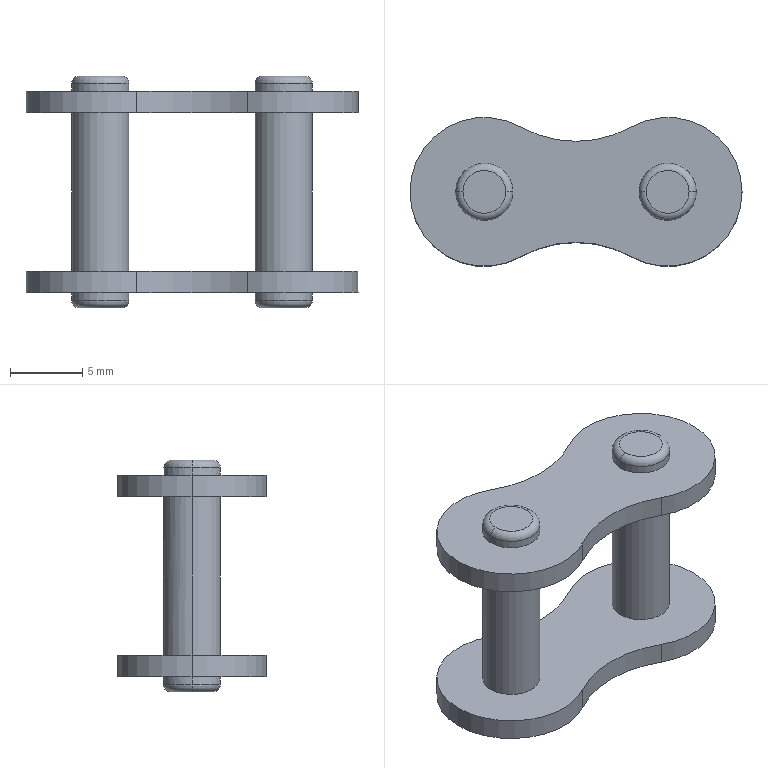Part | STEP file | _CHE40-500_c1 | 1 solid | 40 faces | box 23 x 10.3 x 16.04 mm | volume 895.191 mm3 | cylinder 24 | plane 8 | torus 8 | commonest cylinder face diameters 3.97 x12 10.3 x8 15.788 x4
STEP:
#1=CARTESIAN_POINT('',(2.507,4.499,-5.475));
#2=VERTEX_POINT('',#1);
#3=CARTESIAN_POINT('',(10.193,4.499,-5.475));
#4=VERTEX_POINT('',#3);
#5=CARTESIAN_POINT('',(6.35,11.394,-5.475));
#6=DIRECTION('',(0.,0.,1.));
#7=AXIS2_PLACEMENT_3D('',#5,#6,$);
#8=CIRCLE('',#7,7.894);
#9=EDGE_CURVE('',#2,#4,#8,.T.);
#10=ORIENTED_EDGE('',*,*,#9,.F.);
#11=CARTESIAN_POINT('',(-5.15,0.,-5.475));
#12=VERTEX_POINT('',#11);
#13=CARTESIAN_POINT('',(0.,0.,-5.475));
#14=DIRECTION('',(0.,0.,1.));
#15=AXIS2_PLACEMENT_3D('',#13,#14,$);
#16=CIRCLE('',#15,5.15);
#17=EDGE_CURVE('',#2,#12,#16,.T.);
#18=ORIENTED_EDGE('',*,*,#17,.T.);
#19=CARTESIAN_POINT('',(2.507,-4.499,-5.475));
#20=VERTEX_POINT('',#19);
#21=CARTESIAN_POINT('',(0.,0.,-5.475));
#22=DIRECTION('',(0.,0.,1.));
#23=AXIS2_PLACEMENT_3D('',#21,#22,$);
#24=CIRCLE('',#23,5.15);
#25=EDGE_CURVE('',#12,#20,#24,.T.);
#26=ORIENTED_EDGE('',*,*,#25,.T.);
#27=CARTESIAN_POINT('',(10.193,-4.499,-5.475));
#28=VERTEX_POINT('',#27);
#29=CARTESIAN_POINT('',(6.35,-11.394,-5.475));
#30=DIRECTION('',(0.,0.,1.));
#31=AXIS2_PLACEMENT_3D('',#29,#30,$);
#32=CIRCLE('',#31,7.894);
#33=EDGE_CURVE('',#28,#20,#32,.T.);
#34=ORIENTED_EDGE('',*,*,#33,.F.);
#35=CARTESIAN_POINT('',(17.85,0.,-5.475));
#36=VERTEX_POINT('',#35);
#37=CARTESIAN_POINT('',(12.7,0.,-5.475));
#38=DIRECTION('',(0.,0.,1.));
#39=AXIS2_PLACEMENT_3D('',#37,#38,$);
#40=CIRCLE('',#39,5.15);
#41=EDGE_CURVE('',#28,#36,#40,.T.);
#42=ORIENTED_EDGE('',*,*,#41,.T.);
#43=CARTESIAN_POINT('',(12.7,0.,-5.475));
#44=DIRECTION('',(0.,0.,1.));
#45=AXIS2_PLACEMENT_3D('',#43,#44,$);
#46=CIRCLE('',#45,5.15);
#47=EDGE_CURVE('',#36,#4,#46,.T.);
#48=ORIENTED_EDGE('',*,*,#47,.T.);
#49=EDGE_LOOP('',(#10,#18,#26,#34,#42,#48));
#50=FACE_OUTER_BOUND('',#49,.T.);
#51=CARTESIAN_POINT('',(-1.985,0.000000001,-5.475));
#52=VERTEX_POINT('',#51);
#53=CARTESIAN_POINT('',(1.985,0.000000001,-5.475));
#54=VERTEX_POINT('',#53);
#55=CARTESIAN_POINT('',(0.000000001,0.,-5.475));
#56=DIRECTION('',(0.,0.,1.));
#57=AXIS2_PLACEMENT_3D('',#55,#56,$);
#58=CIRCLE('',#57,1.985);
#59=EDGE_CURVE('',#52,#54,#58,.T.);
#60=ORIENTED_EDGE('',*,*,#59,.F.);
#61=CARTESIAN_POINT('',(0.000000001,0.,-5.475));
#62=DIRECTION('',(0.,0.,1.));
#63=AXIS2_PLACEMENT_3D('',#61,#62,$);
#64=CIRCLE('',#63,1.985);
#65=EDGE_CURVE('',#54,#52,#64,.T.);
#66=ORIENTED_EDGE('',*,*,#65,.F.);
#67=EDGE_LOOP('',(#60,#66));
#68=FACE_BOUND('',#67,.T.);
#69=CARTESIAN_POINT('',(10.715,0.000000001,-5.475));
#70=VERTEX_POINT('',#69);
#71=CARTESIAN_POINT('',(14.685,0.000000001,-5.475));
#72=VERTEX_POINT('',#71);
#73=CARTESIAN_POINT('',(12.7,0.,-5.475));
#74=DIRECTION('',(0.,0.,1.));
#75=AXIS2_PLACEMENT_3D('',#73,#74,$);
#76=CIRCLE('',#75,1.985);
#77=EDGE_CURVE('',#70,#72,#76,.T.);
#78=ORIENTED_EDGE('',*,*,#77,.F.);
#79=CARTESIAN_POINT('',(12.7,0.,-5.475));
#80=DIRECTION('',(0.,0.,1.));
#81=AXIS2_PLACEMENT_3D('',#79,#80,$);
#82=CIRCLE('',#81,1.985);
#83=EDGE_CURVE('',#72,#70,#82,.T.);
#84=ORIENTED_EDGE('',*,*,#83,.F.);
#85=EDGE_LOOP('',(#78,#84));
#86=FACE_BOUND('',#85,.T.);
#87=CARTESIAN_POINT('',(9.525,5.697,-5.475));
#88=DIRECTION('',(0.,0.,1.));
#89=DIRECTION('',(1.,0.,0.));
#90=AXIS2_PLACEMENT_3D('',#87,#88,#89);
#91=PLANE('',#90);
#92=ADVANCED_FACE('',(#50,#68,#86),#91,.T.);
#93=ORIENTED_EDGE('',*,*,#9,.T.);
#94=CARTESIAN_POINT('',(10.193,4.499,-6.975));
#95=VERTEX_POINT('',#94);
#96=CARTESIAN_POINT('',(10.193,4.499,-6.975));
#97=DIRECTION('',(0.,0.,-1.));
#98=VECTOR('',#97,1.);
#99=LINE('',#96,#98);
#100=EDGE_CURVE('',#95,#4,#99,.F.);
#101=ORIENTED_EDGE('',*,*,#100,.F.);
#102=CARTESIAN_POINT('',(2.507,4.499,-6.975));
#103=VERTEX_POINT('',#102);
#104=CARTESIAN_POINT('',(6.35,11.394,-6.975));
#105=DIRECTION('',(0.,0.,-1.));
#106=AXIS2_PLACEMENT_3D('',#104,#105,$);
#107=CIRCLE('',#106,7.894);
#108=EDGE_CURVE('',#103,#95,#107,.F.);
#109=ORIENTED_EDGE('',*,*,#108,.F.);
#110=CARTESIAN_POINT('',(2.507,4.499,-6.975));
#111=DIRECTION('',(0.,0.,-1.));
#112=VECTOR('',#111,1.);
#113=LINE('',#110,#112);
#114=EDGE_CURVE('',#103,#2,#113,.F.);
#115=ORIENTED_EDGE('',*,*,#114,.T.);
#116=EDGE_LOOP('',(#93,#101,#109,#115));
#117=FACE_OUTER_BOUND('',#116,.T.);
#118=CARTESIAN_POINT('',(6.35,11.394,-6.975));
#119=DIRECTION('',(0.,0.,-1.));
#120=DIRECTION('',(1.,0.,0.));
#121=AXIS2_PLACEMENT_3D('',#118,#119,#120);
#122=CYLINDRICAL_SURFACE('',#121,7.894);
#123=ADVANCED_FACE('',(#117),#122,.F.);
#124=CARTESIAN_POINT('',(-5.15,0.,-6.975));
#125=VERTEX_POINT('',#124);
#126=CARTESIAN_POINT('',(-5.15,0.,-6.975));
#127=DIRECTION('',(0.,0.,-1.));
#128=VECTOR('',#127,1.);
#129=LINE('',#126,#128);
#130=EDGE_CURVE('',#12,#125,#129,.T.);
#131=ORIENTED_EDGE('',*,*,#130,.F.);
#132=ORIENTED_EDGE('',*,*,#17,.F.);
#133=ORIENTED_EDGE('',*,*,#114,.F.);
#134=CARTESIAN_POINT('',(0.,0.,-6.975));
#135=DIRECTION('',(0.,0.,-1.));
#136=AXIS2_PLACEMENT_3D('',#134,#135,$);
#137=CIRCLE('',#136,5.15);
#138=EDGE_CURVE('',#103,#125,#137,.F.);
#139=ORIENTED_EDGE('',*,*,#138,.T.);
#140=EDGE_LOOP('',(#131,#132,#133,#139));
#141=FACE_OUTER_BOUND('',#140,.T.);
#142=CARTESIAN_POINT('',(0.,0.,-6.975));
#143=DIRECTION('',(0.,0.,-1.));
#144=DIRECTION('',(-1.,0.,0.));
#145=AXIS2_PLACEMENT_3D('',#142,#143,#144);
#146=CYLINDRICAL_SURFACE('',#145,5.15);
#147=ADVANCED_FACE('',(#141),#146,.T.);
#148=ORIENTED_EDGE('',*,*,#130,.T.);
#149=CARTESIAN_POINT('',(2.507,-4.499,-6.975));
#150=VERTEX_POINT('',#149);
#151=CARTESIAN_POINT('',(0.,0.,-6.975));
#152=DIRECTION('',(0.,0.,-1.));
#153=AXIS2_PLACEMENT_3D('',#151,#152,$);
#154=CIRCLE('',#153,5.15);
#155=EDGE_CURVE('',#125,#150,#154,.F.);
#156=ORIENTED_EDGE('',*,*,#155,.T.);
#157=CARTESIAN_POINT('',(2.507,-4.499,-6.975));
#158=DIRECTION('',(0.,0.,-1.));
#159=VECTOR('',#158,1.);
#160=LINE('',#157,#159);
#161=EDGE_CURVE('',#150,#20,#160,.F.);
#162=ORIENTED_EDGE('',*,*,#161,.T.);
#163=ORIENTED_EDGE('',*,*,#25,.F.);
#164=EDGE_LOOP('',(#148,#156,#162,#163));
#165=FACE_OUTER_BOUND('',#164,.T.);
#166=CARTESIAN_POINT('',(0.,0.,-6.975));
#167=DIRECTION('',(0.,0.,-1.));
#168=DIRECTION('',(1.,0.,0.));
#169=AXIS2_PLACEMENT_3D('',#166,#167,#168);
#170=CYLINDRICAL_SURFACE('',#169,5.15);
#171=ADVANCED_FACE('',(#165),#170,.T.);
#172=ORIENTED_EDGE('',*,*,#33,.T.);
#173=ORIENTED_EDGE('',*,*,#161,.F.);
#174=CARTESIAN_POINT('',(10.193,-4.499,-6.975));
#175=VERTEX_POINT('',#174);
#176=CARTESIAN_POINT('',(6.35,-11.394,-6.975));
#177=DIRECTION('',(0.,0.,-1.));
#178=AXIS2_PLACEMENT_3D('',#176,#177,$);
#179=CIRCLE('',#178,7.894);
#180=EDGE_CURVE('',#175,#150,#179,.F.);
#181=ORIENTED_EDGE('',*,*,#180,.F.);
#182=CARTESIAN_POINT('',(10.193,-4.499,-6.975));
#183=DIRECTION('',(0.,0.,-1.));
#184=VECTOR('',#183,1.);
#185=LINE('',#182,#184);
#186=EDGE_CURVE('',#175,#28,#185,.F.);
#187=ORIENTED_EDGE('',*,*,#186,.T.);
#188=EDGE_LOOP('',(#172,#173,#181,#187));
#189=FACE_OUTER_BOUND('',#188,.T.);
#190=CARTESIAN_POINT('',(6.35,-11.394,-6.975));
#191=DIRECTION('',(0.,0.,-1.));
#192=DIRECTION('',(-1.,0.,0.));
#193=AXIS2_PLACEMENT_3D('',#190,#191,#192);
#194=CYLINDRICAL_SURFACE('',#193,7.894);
#195=ADVANCED_FACE('',(#189),#194,.F.);
#196=CARTESIAN_POINT('',(17.85,0.,-6.975));
#197=VERTEX_POINT('',#196);
#198=CARTESIAN_POINT('',(17.85,0.,-6.975));
#199=DIRECTION('',(0.,0.,-1.));
#200=VECTOR('',#199,1.);
#201=LINE('',#198,#200);
#202=EDGE_CURVE('',#197,#36,#201,.F.);
#203=ORIENTED_EDGE('',*,*,#202,.T.);
#204=ORIENTED_EDGE('',*,*,#41,.F.);
#205=ORIENTED_EDGE('',*,*,#186,.F.);
#206=CARTESIAN_POINT('',(12.7,0.,-6.975));
#207=DIRECTION('',(0.,0.,-1.));
#208=AXIS2_PLACEMENT_3D('',#206,#207,$);
#209=CIRCLE('',#208,5.15);
#210=EDGE_CURVE('',#175,#197,#209,.F.);
#211=ORIENTED_EDGE('',*,*,#210,.T.);
#212=EDGE_LOOP('',(#203,#204,#205,#211));
#213=FACE_OUTER_BOUND('',#212,.T.);
#214=CARTESIAN_POINT('',(12.7,0.,-6.975));
#215=DIRECTION('',(0.,0.,-1.));
#216=DIRECTION('',(1.,0.,0.));
#217=AXIS2_PLACEMENT_3D('',#214,#215,#216);
#218=CYLINDRICAL_SURFACE('',#217,5.15);
#219=ADVANCED_FACE('',(#213),#218,.T.);
#220=ORIENTED_EDGE('',*,*,#202,.F.);
#221=CARTESIAN_POINT('',(12.7,0.,-6.975));
#222=DIRECTION('',(0.,0.,-1.));
#223=AXIS2_PLACEMENT_3D('',#221,#222,$);
#224=CIRCLE('',#223,5.15);
#225=EDGE_CURVE('',#197,#95,#224,.F.);
#226=ORIENTED_EDGE('',*,*,#225,.T.);
#227=ORIENTED_EDGE('',*,*,#100,.T.);
#228=ORIENTED_EDGE('',*,*,#47,.F.);
#229=EDGE_LOOP('',(#220,#226,#227,#228));
#230=FACE_OUTER_BOUND('',#229,.T.);
#231=CARTESIAN_POINT('',(12.7,0.,-6.975));
#232=DIRECTION('',(0.,0.,-1.));
#233=DIRECTION('',(-1.,0.,0.));
#234=AXIS2_PLACEMENT_3D('',#231,#232,#233);
#235=CYLINDRICAL_SURFACE('',#234,5.15);
#236=ADVANCED_FACE('',(#230),#235,.T.);
#237=CARTESIAN_POINT('',(-1.985,0.000000001,5.475));
#238=VERTEX_POINT('',#237);
#239=CARTESIAN_POINT('',(-1.985,0.,8.02));
#240=DIRECTION('',(0.,0.,-1.));
#241=VECTOR('',#240,1.);
#242=LINE('',#239,#241);
#243=EDGE_CURVE('',#238,#52,#242,.T.);
#244=ORIENTED_EDGE('',*,*,#243,.T.);
#245=ORIENTED_EDGE('',*,*,#59,.T.);
#246=CARTESIAN_POINT('',(1.985,0.000000001,5.475));
#247=VERTEX_POINT('',#246);
#248=CARTESIAN_POINT('',(1.985,0.,8.02));
#249=DIRECTION('',(0.,0.,-1.));
#250=VECTOR('',#249,1.);
#251=LINE('',#248,#250);
#252=EDGE_CURVE('',#54,#247,#251,.F.);
#253=ORIENTED_EDGE('',*,*,#252,.T.);
#254=CARTESIAN_POINT('',(0.,0.,5.475));
#255=DIRECTION('',(0.,0.,-1.));
#256=AXIS2_PLACEMENT_3D('',#254,#255,$);
#257=CIRCLE('',#256,1.985);
#258=EDGE_CURVE('',#247,#238,#257,.T.);
#259=ORIENTED_EDGE('',*,*,#258,.T.);
#260=EDGE_LOOP('',(#244,#245,#253,#259));
#261=FACE_OUTER_BOUND('',#260,.T.);
#262=CARTESIAN_POINT('',(0.,0.,8.02));
#263=DIRECTION('',(0.,0.,-1.));
#264=DIRECTION('',(1.,0.,0.));
#265=AXIS2_PLACEMENT_3D('',#262,#263,#264);
#266=CYLINDRICAL_SURFACE('',#265,1.985);
#267=ADVANCED_FACE('',(#261),#266,.T.);
#268=ORIENTED_EDGE('',*,*,#252,.F.);
#269=ORIENTED_EDGE('',*,*,#65,.T.);
#270=ORIENTED_EDGE('',*,*,#243,.F.);
#271=CARTESIAN_POINT('',(1.985,0.,5.475));
#272=CARTESIAN_POINT('',(1.985,0.6236,5.475));
#273=CARTESIAN_POINT('',(1.74,1.247,5.475));
#274=CARTESIAN_POINT('',(1.247,1.74,5.475));
#275=CARTESIAN_POINT('',(0.,2.23,5.475));
#276=CARTESIAN_POINT('',(-1.247,1.74,5.475));
#277=CARTESIAN_POINT('',(-1.74,1.247,5.475));
#278=CARTESIAN_POINT('',(-1.985,0.6236,5.475));
#279=CARTESIAN_POINT('',(-1.985,0.,5.475));
#280=B_SPLINE_CURVE_WITH_KNOTS('',5,(#271,#272,#273,#274,#275,#276,#277,#278,#279),.UNSPECIFIED.,.F.,.U.,(6,3,6),(-3.118,0.,3.118),.UNSPECIFIED.);
#281=EDGE_CURVE('',#238,#247,#280,.F.);
#282=ORIENTED_EDGE('',*,*,#281,.T.);
#283=EDGE_LOOP('',(#268,#269,#270,#282));
#284=FACE_OUTER_BOUND('',#283,.T.);
#285=CARTESIAN_POINT('',(0.,0.,8.02));
#286=DIRECTION('',(0.,0.,-1.));
#287=DIRECTION('',(-1.,0.,0.));
#288=AXIS2_PLACEMENT_3D('',#285,#286,#287);
#289=CYLINDRICAL_SURFACE('',#288,1.985);
#290=ADVANCED_FACE('',(#284),#289,.T.);
#291=CARTESIAN_POINT('',(10.715,0.000000001,5.475));
#292=VERTEX_POINT('',#291);
#293=CARTESIAN_POINT('',(10.715,0.,8.02));
#294=DIRECTION('',(0.,0.,-1.));
#295=VECTOR('',#294,1.);
#296=LINE('',#293,#295);
#297=EDGE_CURVE('',#292,#70,#296,.T.);
#298=ORIENTED_EDGE('',*,*,#297,.T.);
#299=ORIENTED_EDGE('',*,*,#77,.T.);
#300=CARTESIAN_POINT('',(14.685,0.000000001,5.475));
#301=VERTEX_POINT('',#300);
#302=CARTESIAN_POINT('',(14.685,0.,8.02));
#303=DIRECTION('',(0.,0.,-1.));
#304=VECTOR('',#303,1.);
#305=LINE('',#302,#304);
#306=EDGE_CURVE('',#72,#301,#305,.F.);
#307=ORIENTED_EDGE('',*,*,#306,.T.);
#308=CARTESIAN_POINT('',(12.7,0.,5.475));
#309=DIRECTION('',(0.,0.,-1.));
#310=AXIS2_PLACEMENT_3D('',#308,#309,$);
#311=CIRCLE('',#310,1.985);
#312=EDGE_CURVE('',#301,#292,#311,.T.);
#313=ORIENTED_EDGE('',*,*,#312,.T.);
#314=EDGE_LOOP('',(#298,#299,#307,#313));
#315=FACE_OUTER_BOUND('',#314,.T.);
#316=CARTESIAN_POINT('',(12.7,0.,8.02));
#317=DIRECTION('',(0.,0.,-1.));
#318=DIRECTION('',(1.,0.,0.));
#319=AXIS2_PLACEMENT_3D('',#316,#317,#318);
#320=CYLINDRICAL_SURFACE('',#319,1.985);
#321=ADVANCED_FACE('',(#315),#320,.T.);
#322=ORIENTED_EDGE('',*,*,#306,.F.);
#323=ORIENTED_EDGE('',*,*,#83,.T.);
#324=ORIENTED_EDGE('',*,*,#297,.F.);
#325=CARTESIAN_POINT('',(14.685,0.,5.475));
#326=CARTESIAN_POINT('',(14.685,0.6236,5.475));
#327=CARTESIAN_POINT('',(14.44,1.247,5.475));
#328=CARTESIAN_POINT('',(13.947,1.74,5.475));
#329=CARTESIAN_POINT('',(12.7,2.23,5.475));
#330=CARTESIAN_POINT('',(11.453,1.74,5.475));
#331=CARTESIAN_POINT('',(10.96,1.247,5.475));
#332=CARTESIAN_POINT('',(10.715,0.6236,5.475));
#333=CARTESIAN_POINT('',(10.715,0.,5.475));
#334=B_SPLINE_CURVE_WITH_KNOTS('',5,(#325,#326,#327,#328,#329,#330,#331,#332,#333),.UNSPECIFIED.,.F.,.U.,(6,3,6),(-3.118,0.,3.118),.UNSPECIFIED.);
#335=EDGE_CURVE('',#292,#301,#334,.F.);
#336=ORIENTED_EDGE('',*,*,#335,.T.);
#337=EDGE_LOOP('',(#322,#323,#324,#336));
#338=FACE_OUTER_BOUND('',#337,.T.);
#339=CARTESIAN_POINT('',(12.7,0.,8.02));
#340=DIRECTION('',(0.,0.,-1.));
#341=DIRECTION('',(-1.,0.,0.));
#342=AXIS2_PLACEMENT_3D('',#339,#340,#341);
#343=CYLINDRICAL_SURFACE('',#342,1.985);
#344=ADVANCED_FACE('',(#338),#343,.T.);
#345=ORIENTED_EDGE('',*,*,#108,.T.);
#346=ORIENTED_EDGE('',*,*,#225,.F.);
#347=ORIENTED_EDGE('',*,*,#210,.F.);
#348=ORIENTED_EDGE('',*,*,#180,.T.);
#349=ORIENTED_EDGE('',*,*,#155,.F.);
#350=ORIENTED_EDGE('',*,*,#138,.F.);
#351=EDGE_LOOP('',(#345,#346,#347,#348,#349,#350));
#352=FACE_OUTER_BOUND('',#351,.T.);
#353=CARTESIAN_POINT('',(1.985,0.,-6.975));
#354=VERTEX_POINT('',#353);
#355=CARTESIAN_POINT('',(-1.985,0.,-6.975));
#356=VERTEX_POINT('',#355);
#357=CARTESIAN_POINT('',(0.000000001,0.,-6.975));
#358=DIRECTION('',(0.,0.,1.));
#359=AXIS2_PLACEMENT_3D('',#357,#358,$);
#360=CIRCLE('',#359,1.985);
#361=EDGE_CURVE('',#354,#356,#360,.T.);
#362=ORIENTED_EDGE('',*,*,#361,.T.);
#363=CARTESIAN_POINT('',(0.000000001,0.,-6.975));
#364=DIRECTION('',(0.,0.,1.));
#365=AXIS2_PLACEMENT_3D('',#363,#364,$);
#366=CIRCLE('',#365,1.985);
#367=EDGE_CURVE('',#356,#354,#366,.T.);
#368=ORIENTED_EDGE('',*,*,#367,.T.);
#369=EDGE_LOOP('',(#362,#368));
#370=FACE_BOUND('',#369,.T.);
#371=CARTESIAN_POINT('',(14.685,0.000000001,-6.975));
#372=VERTEX_POINT('',#371);
#373=CARTESIAN_POINT('',(10.715,0.000000001,-6.975));
#374=VERTEX_POINT('',#373);
#375=CARTESIAN_POINT('',(12.7,0.,-6.975));
#376=DIRECTION('',(0.,0.,1.));
#377=AXIS2_PLACEMENT_3D('',#375,#376,$);
#378=CIRCLE('',#377,1.985);
#379=EDGE_CURVE('',#372,#374,#378,.T.);
#380=ORIENTED_EDGE('',*,*,#379,.T.);
#381=CARTESIAN_POINT('',(12.7,0.,-6.975));
#382=DIRECTION('',(0.,0.,1.));
#383=AXIS2_PLACEMENT_3D('',#381,#382,$);
#384=CIRCLE('',#383,1.985);
#385=EDGE_CURVE('',#374,#372,#384,.T.);
#386=ORIENTED_EDGE('',*,*,#385,.T.);
#387=EDGE_LOOP('',(#380,#386));
#388=FACE_BOUND('',#387,.T.);
#389=CARTESIAN_POINT('',(9.525,5.697,-6.975));
#390=DIRECTION('',(0.,0.,1.));
#391=DIRECTION('',(1.,0.,0.));
#392=AXIS2_PLACEMENT_3D('',#389,#390,#391);
#393=PLANE('',#392);
#394=ADVANCED_FACE('',(#352,#370,#388),#393,.F.);
#395=CARTESIAN_POINT('',(2.507,4.499,5.475));
#396=VERTEX_POINT('',#395);
#397=CARTESIAN_POINT('',(10.193,4.499,5.475));
#398=VERTEX_POINT('',#397);
#399=CARTESIAN_POINT('',(6.35,11.394,5.475));
#400=DIRECTION('',(0.,0.,1.));
#401=AXIS2_PLACEMENT_3D('',#399,#400,$);
#402=CIRCLE('',#401,7.894);
#403=EDGE_CURVE('',#396,#398,#402,.T.);
#404=ORIENTED_EDGE('',*,*,#403,.T.);
#405=CARTESIAN_POINT('',(17.85,0.,5.475));
#406=VERTEX_POINT('',#405);
#407=CARTESIAN_POINT('',(12.7,0.,5.475));
#408=DIRECTION('',(0.,0.,1.));
#409=AXIS2_PLACEMENT_3D('',#407,#408,$);
#410=CIRCLE('',#409,5.15);
#411=EDGE_CURVE('',#406,#398,#410,.T.);
#412=ORIENTED_EDGE('',*,*,#411,.F.);
#413=CARTESIAN_POINT('',(10.193,-4.499,5.475));
#414=VERTEX_POINT('',#413);
#415=CARTESIAN_POINT('',(12.7,0.,5.475));
#416=DIRECTION('',(0.,0.,1.));
#417=AXIS2_PLACEMENT_3D('',#415,#416,$);
#418=CIRCLE('',#417,5.15);
#419=EDGE_CURVE('',#414,#406,#418,.T.);
#420=ORIENTED_EDGE('',*,*,#419,.F.);
#421=CARTESIAN_POINT('',(2.507,-4.499,5.475));
#422=VERTEX_POINT('',#421);
#423=CARTESIAN_POINT('',(6.35,-11.394,5.475));
#424=DIRECTION('',(0.,0.,1.));
#425=AXIS2_PLACEMENT_3D('',#423,#424,$);
#426=CIRCLE('',#425,7.894);
#427=EDGE_CURVE('',#414,#422,#426,.T.);
#428=ORIENTED_EDGE('',*,*,#427,.T.);
#429=CARTESIAN_POINT('',(-5.15,0.,5.475));
#430=VERTEX_POINT('',#429);
#431=CARTESIAN_POINT('',(0.,0.,5.475));
#432=DIRECTION('',(0.,0.,1.));
#433=AXIS2_PLACEMENT_3D('',#431,#432,$);
#434=CIRCLE('',#433,5.15);
#435=EDGE_CURVE('',#430,#422,#434,.T.);
#436=ORIENTED_EDGE('',*,*,#435,.F.);
#437=CARTESIAN_POINT('',(0.,0.,5.475));
#438=DIRECTION('',(0.,0.,1.));
#439=AXIS2_PLACEMENT_3D('',#437,#438,$);
#440=CIRCLE('',#439,5.15);
#441=EDGE_CURVE('',#396,#430,#440,.T.);
#442=ORIENTED_EDGE('',*,*,#441,.F.);
#443=EDGE_LOOP('',(#404,#412,#420,#428,#436,#442));
#444=FACE_OUTER_BOUND('',#443,.T.);
#445=ORIENTED_EDGE('',*,*,#335,.F.);
#446=ORIENTED_EDGE('',*,*,#312,.F.);
#447=EDGE_LOOP('',(#445,#446));
#448=FACE_BOUND('',#447,.T.);
#449=ORIENTED_EDGE('',*,*,#281,.F.);
#450=ORIENTED_EDGE('',*,*,#258,.F.);
#451=EDGE_LOOP('',(#449,#450));
#452=FACE_BOUND('',#451,.T.);
#453=CARTESIAN_POINT('',(9.525,5.697,5.475));
#454=DIRECTION('',(0.,0.,1.));
#455=DIRECTION('',(1.,0.,0.));
#456=AXIS2_PLACEMENT_3D('',#453,#454,#455);
#457=PLANE('',#456);
#458=ADVANCED_FACE('',(#444,#448,#452),#457,.F.);
#459=CARTESIAN_POINT('',(1.985,0.,-7.52));
#460=VERTEX_POINT('',#459);
#461=CARTESIAN_POINT('',(1.985,0.,8.02));
#462=DIRECTION('',(0.,0.,-1.));
#463=VECTOR('',#462,1.);
#464=LINE('',#461,#463);
#465=EDGE_CURVE('',#460,#354,#464,.F.);
#466=ORIENTED_EDGE('',*,*,#465,.F.);
#467=CARTESIAN_POINT('',(-1.985,0.,-7.52));
#468=VERTEX_POINT('',#467);
#469=CARTESIAN_POINT('',(1.985,0.,-7.52));
#470=CARTESIAN_POINT('',(1.985,0.6236,-7.52));
#471=CARTESIAN_POINT('',(1.74,1.247,-7.52));
#472=CARTESIAN_POINT('',(1.247,1.74,-7.52));
#473=CARTESIAN_POINT('',(0.,2.23,-7.52));
#474=CARTESIAN_POINT('',(-1.247,1.74,-7.52));
#475=CARTESIAN_POINT('',(-1.74,1.247,-7.52));
#476=CARTESIAN_POINT('',(-1.985,0.6236,-7.52));
#477=CARTESIAN_POINT('',(-1.985,0.,-7.52));
#478=B_SPLINE_CURVE_WITH_KNOTS('',5,(#469,#470,#471,#472,#473,#474,#475,#476,#477),.UNSPECIFIED.,.F.,.U.,(6,3,6),(-3.118,0.,3.118),.UNSPECIFIED.);
#479=EDGE_CURVE('',#460,#468,#478,.T.);
#480=ORIENTED_EDGE('',*,*,#479,.T.);
#481=CARTESIAN_POINT('',(-1.985,0.,8.02));
#482=DIRECTION('',(0.,0.,-1.));
#483=VECTOR('',#482,1.);
#484=LINE('',#481,#483);
#485=EDGE_CURVE('',#356,#468,#484,.T.);
#486=ORIENTED_EDGE('',*,*,#485,.F.);
#487=ORIENTED_EDGE('',*,*,#361,.F.);
#488=EDGE_LOOP('',(#466,#480,#486,#487));
#489=FACE_OUTER_BOUND('',#488,.T.);
#490=CARTESIAN_POINT('',(0.,0.,8.02));
#491=DIRECTION('',(0.,0.,-1.));
#492=DIRECTION('',(-1.,0.,0.));
#493=AXIS2_PLACEMENT_3D('',#490,#491,#492);
#494=CYLINDRICAL_SURFACE('',#493,1.985);
#495=ADVANCED_FACE('',(#489),#494,.T.);
#496=ORIENTED_EDGE('',*,*,#485,.T.);
#497=CARTESIAN_POINT('',(0.,0.,-7.52));
#498=DIRECTION('',(0.,0.,-1.));
#499=AXIS2_PLACEMENT_3D('',#497,#498,$);
#500=CIRCLE('',#499,1.985);
#501=EDGE_CURVE('',#468,#460,#500,.F.);
#502=ORIENTED_EDGE('',*,*,#501,.T.);
#503=ORIENTED_EDGE('',*,*,#465,.T.);
#504=ORIENTED_EDGE('',*,*,#367,.F.);
#505=EDGE_LOOP('',(#496,#502,#503,#504));
#506=FACE_OUTER_BOUND('',#505,.T.);
#507=CARTESIAN_POINT('',(0.,0.,8.02));
#508=DIRECTION('',(0.,0.,-1.));
#509=DIRECTION('',(1.,0.,0.));
#510=AXIS2_PLACEMENT_3D('',#507,#508,#509);
#511=CYLINDRICAL_SURFACE('',#510,1.985);
#512=ADVANCED_FACE('',(#506),#511,.T.);
#513=CARTESIAN_POINT('',(14.685,0.,-7.52));
#514=VERTEX_POINT('',#513);
#515=CARTESIAN_POINT('',(14.685,0.,8.02));
#516=DIRECTION('',(0.,0.,-1.));
#517=VECTOR('',#516,1.);
#518=LINE('',#515,#517);
#519=EDGE_CURVE('',#514,#372,#518,.F.);
#520=ORIENTED_EDGE('',*,*,#519,.F.);
#521=CARTESIAN_POINT('',(10.715,0.,-7.52));
#522=VERTEX_POINT('',#521);
#523=CARTESIAN_POINT('',(14.685,0.,-7.52));
#524=CARTESIAN_POINT('',(14.685,0.6236,-7.52));
#525=CARTESIAN_POINT('',(14.44,1.247,-7.52));
#526=CARTESIAN_POINT('',(13.947,1.74,-7.52));
#527=CARTESIAN_POINT('',(12.7,2.23,-7.52));
#528=CARTESIAN_POINT('',(11.453,1.74,-7.52));
#529=CARTESIAN_POINT('',(10.96,1.247,-7.52));
#530=CARTESIAN_POINT('',(10.715,0.6236,-7.52));
#531=CARTESIAN_POINT('',(10.715,0.,-7.52));
#532=B_SPLINE_CURVE_WITH_KNOTS('',5,(#523,#524,#525,#526,#527,#528,#529,#530,#531),.UNSPECIFIED.,.F.,.U.,(6,3,6),(-3.118,0.,3.118),.UNSPECIFIED.);
#533=EDGE_CURVE('',#514,#522,#532,.T.);
#534=ORIENTED_EDGE('',*,*,#533,.T.);
#535=CARTESIAN_POINT('',(10.715,0.,8.02));
#536=DIRECTION('',(0.,0.,-1.));
#537=VECTOR('',#536,1.);
#538=LINE('',#535,#537);
#539=EDGE_CURVE('',#374,#522,#538,.T.);
#540=ORIENTED_EDGE('',*,*,#539,.F.);
#541=ORIENTED_EDGE('',*,*,#379,.F.);
#542=EDGE_LOOP('',(#520,#534,#540,#541));
#543=FACE_OUTER_BOUND('',#542,.T.);
#544=CARTESIAN_POINT('',(12.7,0.,8.02));
#545=DIRECTION('',(0.,0.,-1.));
#546=DIRECTION('',(-1.,0.,0.));
#547=AXIS2_PLACEMENT_3D('',#544,#545,#546);
#548=CYLINDRICAL_SURFACE('',#547,1.985);
#549=ADVANCED_FACE('',(#543),#548,.T.);
#550=ORIENTED_EDGE('',*,*,#539,.T.);
#551=CARTESIAN_POINT('',(12.7,0.,-7.52));
#552=DIRECTION('',(0.,0.,-1.));
#553=AXIS2_PLACEMENT_3D('',#551,#552,$);
#554=CIRCLE('',#553,1.985);
#555=EDGE_CURVE('',#522,#514,#554,.F.);
#556=ORIENTED_EDGE('',*,*,#555,.T.);
#557=ORIENTED_EDGE('',*,*,#519,.T.);
#558=ORIENTED_EDGE('',*,*,#385,.F.);
#559=EDGE_LOOP('',(#550,#556,#557,#558));
#560=FACE_OUTER_BOUND('',#559,.T.);
#561=CARTESIAN_POINT('',(12.7,0.,8.02));
#562=DIRECTION('',(0.,0.,-1.));
#563=DIRECTION('',(1.,0.,0.));
#564=AXIS2_PLACEMENT_3D('',#561,#562,#563);
#565=CYLINDRICAL_SURFACE('',#564,1.985);
#566=ADVANCED_FACE('',(#560),#565,.T.);
#567=ORIENTED_EDGE('',*,*,#403,.F.);
#568=CARTESIAN_POINT('',(2.507,4.499,6.975));
#569=VERTEX_POINT('',#568);
#570=CARTESIAN_POINT('',(2.507,4.499,6.975));
#571=DIRECTION('',(0.,0.,1.));
#572=VECTOR('',#571,1.);
#573=LINE('',#570,#572);
#574=EDGE_CURVE('',#569,#396,#573,.F.);
#575=ORIENTED_EDGE('',*,*,#574,.F.);
#576=CARTESIAN_POINT('',(10.193,4.499,6.975));
#577=VERTEX_POINT('',#576);
#578=CARTESIAN_POINT('',(6.35,11.394,6.975));
#579=DIRECTION('',(0.,0.,1.));
#580=AXIS2_PLACEMENT_3D('',#578,#579,$);
#581=CIRCLE('',#580,7.894);
#582=EDGE_CURVE('',#569,#577,#581,.T.);
#583=ORIENTED_EDGE('',*,*,#582,.T.);
#584=CARTESIAN_POINT('',(10.193,4.499,6.975));
#585=DIRECTION('',(0.,0.,1.));
#586=VECTOR('',#585,1.);
#587=LINE('',#584,#586);
#588=EDGE_CURVE('',#577,#398,#587,.F.);
#589=ORIENTED_EDGE('',*,*,#588,.T.);
#590=EDGE_LOOP('',(#567,#575,#583,#589));
#591=FACE_OUTER_BOUND('',#590,.T.);
#592=CARTESIAN_POINT('',(6.35,11.394,6.975));
#593=DIRECTION('',(0.,0.,1.));
#594=DIRECTION('',(-1.,0.,0.));
#595=AXIS2_PLACEMENT_3D('',#592,#593,#594);
#596=CYLINDRICAL_SURFACE('',#595,7.894);
#597=ADVANCED_FACE('',(#591),#596,.F.);
#598=CARTESIAN_POINT('',(17.85,0.,6.975));
#599=VERTEX_POINT('',#598);
#600=CARTESIAN_POINT('',(17.85,0.,6.975));
#601=DIRECTION('',(0.,0.,1.));
#602=VECTOR('',#601,1.);
#603=LINE('',#600,#602);
#604=EDGE_CURVE('',#406,#599,#603,.T.);
#605=ORIENTED_EDGE('',*,*,#604,.F.);
#606=ORIENTED_EDGE('',*,*,#411,.T.);
#607=ORIENTED_EDGE('',*,*,#588,.F.);
#608=CARTESIAN_POINT('',(12.7,0.,6.975));
#609=DIRECTION('',(0.,0.,1.));
#610=AXIS2_PLACEMENT_3D('',#608,#609,$);
#611=CIRCLE('',#610,5.15);
#612=EDGE_CURVE('',#599,#577,#611,.T.);
#613=ORIENTED_EDGE('',*,*,#612,.F.);
#614=EDGE_LOOP('',(#605,#606,#607,#613));
#615=FACE_OUTER_BOUND('',#614,.T.);
#616=CARTESIAN_POINT('',(12.7,0.,6.975));
#617=DIRECTION('',(0.,0.,1.));
#618=DIRECTION('',(1.,0.,0.));
#619=AXIS2_PLACEMENT_3D('',#616,#617,#618);
#620=CYLINDRICAL_SURFACE('',#619,5.15);
#621=ADVANCED_FACE('',(#615),#620,.T.);
#622=ORIENTED_EDGE('',*,*,#604,.T.);
#623=CARTESIAN_POINT('',(10.193,-4.499,6.975));
#624=VERTEX_POINT('',#623);
#625=CARTESIAN_POINT('',(12.7,0.,6.975));
#626=DIRECTION('',(0.,0.,1.));
#627=AXIS2_PLACEMENT_3D('',#625,#626,$);
#628=CIRCLE('',#627,5.15);
#629=EDGE_CURVE('',#624,#599,#628,.T.);
#630=ORIENTED_EDGE('',*,*,#629,.F.);
#631=CARTESIAN_POINT('',(10.193,-4.499,6.975));
#632=DIRECTION('',(0.,0.,1.));
#633=VECTOR('',#632,1.);
#634=LINE('',#631,#633);
#635=EDGE_CURVE('',#624,#414,#634,.F.);
#636=ORIENTED_EDGE('',*,*,#635,.T.);
#637=ORIENTED_EDGE('',*,*,#419,.T.);
#638=EDGE_LOOP('',(#622,#630,#636,#637));
#639=FACE_OUTER_BOUND('',#638,.T.);
#640=CARTESIAN_POINT('',(12.7,0.,6.975));
#641=DIRECTION('',(0.,0.,1.));
#642=DIRECTION('',(-1.,0.,0.));
#643=AXIS2_PLACEMENT_3D('',#640,#641,#642);
#644=CYLINDRICAL_SURFACE('',#643,5.15);
#645=ADVANCED_FACE('',(#639),#644,.T.);
#646=ORIENTED_EDGE('',*,*,#427,.F.);
#647=ORIENTED_EDGE('',*,*,#635,.F.);
#648=CARTESIAN_POINT('',(2.507,-4.499,6.975));
#649=VERTEX_POINT('',#648);
#650=CARTESIAN_POINT('',(6.35,-11.394,6.975));
#651=DIRECTION('',(0.,0.,1.));
#652=AXIS2_PLACEMENT_3D('',#650,#651,$);
#653=CIRCLE('',#652,7.894);
#654=EDGE_CURVE('',#624,#649,#653,.T.);
#655=ORIENTED_EDGE('',*,*,#654,.T.);
#656=CARTESIAN_POINT('',(2.507,-4.499,6.975));
#657=DIRECTION('',(0.,0.,1.));
#658=VECTOR('',#657,1.);
#659=LINE('',#656,#658);
#660=EDGE_CURVE('',#649,#422,#659,.F.);
#661=ORIENTED_EDGE('',*,*,#660,.T.);
#662=EDGE_LOOP('',(#646,#647,#655,#661));
#663=FACE_OUTER_BOUND('',#662,.T.);
#664=CARTESIAN_POINT('',(6.35,-11.394,6.975));
#665=DIRECTION('',(0.,0.,1.));
#666=DIRECTION('',(1.,0.,0.));
#667=AXIS2_PLACEMENT_3D('',#664,#665,#666);
#668=CYLINDRICAL_SURFACE('',#667,7.894);
#669=ADVANCED_FACE('',(#663),#668,.F.);
#670=CARTESIAN_POINT('',(-5.15,0.,6.975));
#671=VERTEX_POINT('',#670);
#672=CARTESIAN_POINT('',(-5.15,0.,6.975));
#673=DIRECTION('',(0.,0.,1.));
#674=VECTOR('',#673,1.);
#675=LINE('',#672,#674);
#676=EDGE_CURVE('',#671,#430,#675,.F.);
#677=ORIENTED_EDGE('',*,*,#676,.T.);
#678=ORIENTED_EDGE('',*,*,#435,.T.);
#679=ORIENTED_EDGE('',*,*,#660,.F.);
#680=CARTESIAN_POINT('',(0.,0.,6.975));
#681=DIRECTION('',(0.,0.,1.));
#682=AXIS2_PLACEMENT_3D('',#680,#681,$);
#683=CIRCLE('',#682,5.15);
#684=EDGE_CURVE('',#671,#649,#683,.T.);
#685=ORIENTED_EDGE('',*,*,#684,.F.);
#686=EDGE_LOOP('',(#677,#678,#679,#685));
#687=FACE_OUTER_BOUND('',#686,.T.);
#688=CARTESIAN_POINT('',(0.,0.,6.975));
#689=DIRECTION('',(0.,0.,1.));
#690=DIRECTION('',(-1.,0.,0.));
#691=AXIS2_PLACEMENT_3D('',#688,#689,#690);
#692=CYLINDRICAL_SURFACE('',#691,5.15);
#693=ADVANCED_FACE('',(#687),#692,.T.);
#694=ORIENTED_EDGE('',*,*,#676,.F.);
#695=CARTESIAN_POINT('',(0.,0.,6.975));
#696=DIRECTION('',(0.,0.,1.));
#697=AXIS2_PLACEMENT_3D('',#695,#696,$);
#698=CIRCLE('',#697,5.15);
#699=EDGE_CURVE('',#569,#671,#698,.T.);
#700=ORIENTED_EDGE('',*,*,#699,.F.);
#701=ORIENTED_EDGE('',*,*,#574,.T.);
#702=ORIENTED_EDGE('',*,*,#441,.T.);
#703=EDGE_LOOP('',(#694,#700,#701,#702));
#704=FACE_OUTER_BOUND('',#703,.T.);
#705=CARTESIAN_POINT('',(0.,0.,6.975));
#706=DIRECTION('',(0.,0.,1.));
#707=DIRECTION('',(1.,0.,0.));
#708=AXIS2_PLACEMENT_3D('',#705,#706,#707);
#709=CYLINDRICAL_SURFACE('',#708,5.15);
#710=ADVANCED_FACE('',(#704),#709,.T.);
#711=CARTESIAN_POINT('',(-1.485,0.,-8.02));
#712=VERTEX_POINT('',#711);
#713=CARTESIAN_POINT('',(-1.485,0.,-7.52));
#714=DIRECTION('',(0.,1.,0.));
#715=AXIS2_PLACEMENT_3D('',#713,#714,$);
#716=CIRCLE('',#715,0.5);
#717=EDGE_CURVE('',#712,#468,#716,.T.);
#718=ORIENTED_EDGE('',*,*,#717,.T.);
#719=ORIENTED_EDGE('',*,*,#479,.F.);
#720=CARTESIAN_POINT('',(1.485,0.,-8.02));
#721=VERTEX_POINT('',#720);
#722=CARTESIAN_POINT('',(1.485,0.,-7.52));
#723=DIRECTION('',(0.,-1.,0.));
#724=AXIS2_PLACEMENT_3D('',#722,#723,$);
#725=CIRCLE('',#724,0.5);
#726=EDGE_CURVE('',#460,#721,#725,.F.);
#727=ORIENTED_EDGE('',*,*,#726,.T.);
#728=CARTESIAN_POINT('',(0.,0.,-8.02));
#729=DIRECTION('',(0.,0.,1.));
#730=AXIS2_PLACEMENT_3D('',#728,#729,$);
#731=CIRCLE('',#730,1.485);
#732=EDGE_CURVE('',#721,#712,#731,.T.);
#733=ORIENTED_EDGE('',*,*,#732,.T.);
#734=EDGE_LOOP('',(#718,#719,#727,#733));
#735=FACE_OUTER_BOUND('',#734,.T.);
#736=CARTESIAN_POINT('',(0.,0.,-7.52));
#737=DIRECTION('',(0.,0.,1.));
#738=DIRECTION('',(1.,0.,0.));
#739=AXIS2_PLACEMENT_3D('',#736,#737,#738);
#740=TOROIDAL_SURFACE('',#739,1.485,0.5);
#741=ADVANCED_FACE('',(#735),#740,.T.);
#742=ORIENTED_EDGE('',*,*,#726,.F.);
#743=ORIENTED_EDGE('',*,*,#501,.F.);
#744=ORIENTED_EDGE('',*,*,#717,.F.);
#745=CARTESIAN_POINT('',(0.,0.,-8.02));
#746=DIRECTION('',(0.,0.,1.));
#747=AXIS2_PLACEMENT_3D('',#745,#746,$);
#748=CIRCLE('',#747,1.485);
#749=EDGE_CURVE('',#712,#721,#748,.T.);
#750=ORIENTED_EDGE('',*,*,#749,.T.);
#751=EDGE_LOOP('',(#742,#743,#744,#750));
#752=FACE_OUTER_BOUND('',#751,.T.);
#753=CARTESIAN_POINT('',(0.,0.,-7.52));
#754=DIRECTION('',(0.,0.,1.));
#755=DIRECTION('',(-1.,0.,0.));
#756=AXIS2_PLACEMENT_3D('',#753,#754,#755);
#757=TOROIDAL_SURFACE('',#756,1.485,0.5);
#758=ADVANCED_FACE('',(#752),#757,.T.);
#759=CARTESIAN_POINT('',(11.215,0.,-8.02));
#760=VERTEX_POINT('',#759);
#761=CARTESIAN_POINT('',(11.215,0.,-7.52));
#762=DIRECTION('',(0.,1.,0.));
#763=AXIS2_PLACEMENT_3D('',#761,#762,$);
#764=CIRCLE('',#763,0.5);
#765=EDGE_CURVE('',#760,#522,#764,.T.);
#766=ORIENTED_EDGE('',*,*,#765,.T.);
#767=ORIENTED_EDGE('',*,*,#533,.F.);
#768=CARTESIAN_POINT('',(14.185,0.,-8.02));
#769=VERTEX_POINT('',#768);
#770=CARTESIAN_POINT('',(14.185,0.,-7.52));
#771=DIRECTION('',(0.,-1.,0.));
#772=AXIS2_PLACEMENT_3D('',#770,#771,$);
#773=CIRCLE('',#772,0.5);
#774=EDGE_CURVE('',#514,#769,#773,.F.);
#775=ORIENTED_EDGE('',*,*,#774,.T.);
#776=CARTESIAN_POINT('',(12.7,0.,-8.02));
#777=DIRECTION('',(0.,0.,1.));
#778=AXIS2_PLACEMENT_3D('',#776,#777,$);
#779=CIRCLE('',#778,1.485);
#780=EDGE_CURVE('',#769,#760,#779,.T.);
#781=ORIENTED_EDGE('',*,*,#780,.T.);
#782=EDGE_LOOP('',(#766,#767,#775,#781));
#783=FACE_OUTER_BOUND('',#782,.T.);
#784=CARTESIAN_POINT('',(12.7,0.,-7.52));
#785=DIRECTION('',(0.,0.,1.));
#786=DIRECTION('',(1.,0.,0.));
#787=AXIS2_PLACEMENT_3D('',#784,#785,#786);
#788=TOROIDAL_SURFACE('',#787,1.485,0.5);
#789=ADVANCED_FACE('',(#783),#788,.T.);
#790=ORIENTED_EDGE('',*,*,#774,.F.);
#791=ORIENTED_EDGE('',*,*,#555,.F.);
#792=ORIENTED_EDGE('',*,*,#765,.F.);
#793=CARTESIAN_POINT('',(12.7,0.,-8.02));
#794=DIRECTION('',(0.,0.,1.));
#795=AXIS2_PLACEMENT_3D('',#793,#794,$);
#796=CIRCLE('',#795,1.485);
#797=EDGE_CURVE('',#760,#769,#796,.T.);
#798=ORIENTED_EDGE('',*,*,#797,.T.);
#799=EDGE_LOOP('',(#790,#791,#792,#798));
#800=FACE_OUTER_BOUND('',#799,.T.);
#801=CARTESIAN_POINT('',(12.7,0.,-7.52));
#802=DIRECTION('',(0.,0.,1.));
#803=DIRECTION('',(-1.,0.,0.));
#804=AXIS2_PLACEMENT_3D('',#801,#802,#803);
#805=TOROIDAL_SURFACE('',#804,1.485,0.5);
#806=ADVANCED_FACE('',(#800),#805,.T.);
#807=ORIENTED_EDGE('',*,*,#582,.F.);
#808=ORIENTED_EDGE('',*,*,#699,.T.);
#809=ORIENTED_EDGE('',*,*,#684,.T.);
#810=ORIENTED_EDGE('',*,*,#654,.F.);
#811=ORIENTED_EDGE('',*,*,#629,.T.);
#812=ORIENTED_EDGE('',*,*,#612,.T.);
#813=EDGE_LOOP('',(#807,#808,#809,#810,#811,#812));
#814=FACE_OUTER_BOUND('',#813,.T.);
#815=CARTESIAN_POINT('',(14.685,0.000000001,6.975));
#816=VERTEX_POINT('',#815);
#817=CARTESIAN_POINT('',(10.715,0.000000001,6.975));
#818=VERTEX_POINT('',#817);
#819=CARTESIAN_POINT('',(12.7,0.,6.975));
#820=DIRECTION('',(0.,0.,1.));
#821=AXIS2_PLACEMENT_3D('',#819,#820,$);
#822=CIRCLE('',#821,1.985);
#823=EDGE_CURVE('',#816,#818,#822,.F.);
#824=ORIENTED_EDGE('',*,*,#823,.T.);
#825=CARTESIAN_POINT('',(12.7,0.,6.975));
#826=DIRECTION('',(0.,0.,1.));
#827=AXIS2_PLACEMENT_3D('',#825,#826,$);
#828=CIRCLE('',#827,1.985);
#829=EDGE_CURVE('',#818,#816,#828,.F.);
#830=ORIENTED_EDGE('',*,*,#829,.T.);
#831=EDGE_LOOP('',(#824,#830));
#832=FACE_BOUND('',#831,.T.);
#833=CARTESIAN_POINT('',(1.985,0.000000001,6.975));
#834=VERTEX_POINT('',#833);
#835=CARTESIAN_POINT('',(-1.985,0.000000001,6.975));
#836=VERTEX_POINT('',#835);
#837=CARTESIAN_POINT('',(0.000000001,0.,6.975));
#838=DIRECTION('',(0.,0.,1.));
#839=AXIS2_PLACEMENT_3D('',#837,#838,$);
#840=CIRCLE('',#839,1.985);
#841=EDGE_CURVE('',#834,#836,#840,.F.);
#842=ORIENTED_EDGE('',*,*,#841,.T.);
#843=CARTESIAN_POINT('',(0.000000001,0.,6.975));
#844=DIRECTION('',(0.,0.,1.));
#845=AXIS2_PLACEMENT_3D('',#843,#844,$);
#846=CIRCLE('',#845,1.985);
#847=EDGE_CURVE('',#836,#834,#846,.F.);
#848=ORIENTED_EDGE('',*,*,#847,.T.);
#849=EDGE_LOOP('',(#842,#848));
#850=FACE_BOUND('',#849,.T.);
#851=CARTESIAN_POINT('',(9.525,5.697,6.975));
#852=DIRECTION('',(0.,0.,1.));
#853=DIRECTION('',(1.,0.,0.));
#854=AXIS2_PLACEMENT_3D('',#851,#852,#853);
#855=PLANE('',#854);
#856=ADVANCED_FACE('',(#814,#832,#850),#855,.T.);
#857=ORIENTED_EDGE('',*,*,#749,.F.);
#858=ORIENTED_EDGE('',*,*,#732,.F.);
#859=EDGE_LOOP('',(#857,#858));
#860=FACE_OUTER_BOUND('',#859,.T.);
#861=CARTESIAN_POINT('',(0.,0.,-8.02));
#862=DIRECTION('',(0.,0.,1.));
#863=DIRECTION('',(1.,0.,0.));
#864=AXIS2_PLACEMENT_3D('',#861,#862,#863);
#865=PLANE('',#864);
#866=ADVANCED_FACE('',(#860),#865,.F.);
#867=ORIENTED_EDGE('',*,*,#797,.F.);
#868=ORIENTED_EDGE('',*,*,#780,.F.);
#869=EDGE_LOOP('',(#867,#868));
#870=FACE_OUTER_BOUND('',#869,.T.);
#871=CARTESIAN_POINT('',(12.7,0.,-8.02));
#872=DIRECTION('',(0.,0.,1.));
#873=DIRECTION('',(1.,0.,0.));
#874=AXIS2_PLACEMENT_3D('',#871,#872,#873);
#875=PLANE('',#874);
#876=ADVANCED_FACE('',(#870),#875,.F.);
#877=CARTESIAN_POINT('',(10.715,0.,7.52));
#878=VERTEX_POINT('',#877);
#879=CARTESIAN_POINT('',(10.715,0.,8.02));
#880=DIRECTION('',(0.,0.,-1.));
#881=VECTOR('',#880,1.);
#882=LINE('',#879,#881);
#883=EDGE_CURVE('',#878,#818,#882,.T.);
#884=ORIENTED_EDGE('',*,*,#883,.T.);
#885=ORIENTED_EDGE('',*,*,#823,.F.);
#886=CARTESIAN_POINT('',(14.685,0.,7.52));
#887=VERTEX_POINT('',#886);
#888=CARTESIAN_POINT('',(14.685,0.,8.02));
#889=DIRECTION('',(0.,0.,-1.));
#890=VECTOR('',#889,1.);
#891=LINE('',#888,#890);
#892=EDGE_CURVE('',#816,#887,#891,.F.);
#893=ORIENTED_EDGE('',*,*,#892,.T.);
#894=CARTESIAN_POINT('',(12.7,0.,7.52));
#895=DIRECTION('',(0.,0.,-1.));
#896=AXIS2_PLACEMENT_3D('',#894,#895,$);
#897=CIRCLE('',#896,1.985);
#898=EDGE_CURVE('',#878,#887,#897,.F.);
#899=ORIENTED_EDGE('',*,*,#898,.F.);
#900=EDGE_LOOP('',(#884,#885,#893,#899));
#901=FACE_OUTER_BOUND('',#900,.T.);
#902=CARTESIAN_POINT('',(12.7,0.,8.02));
#903=DIRECTION('',(0.,0.,-1.));
#904=DIRECTION('',(1.,0.,0.));
#905=AXIS2_PLACEMENT_3D('',#902,#903,#904);
#906=CYLINDRICAL_SURFACE('',#905,1.985);
#907=ADVANCED_FACE('',(#901),#906,.T.);
#908=ORIENTED_EDGE('',*,*,#892,.F.);
#909=ORIENTED_EDGE('',*,*,#829,.F.);
#910=ORIENTED_EDGE('',*,*,#883,.F.);
#911=CARTESIAN_POINT('',(12.7,0.,7.52));
#912=DIRECTION('',(0.,0.,-1.));
#913=AXIS2_PLACEMENT_3D('',#911,#912,$);
#914=CIRCLE('',#913,1.985);
#915=EDGE_CURVE('',#887,#878,#914,.F.);
#916=ORIENTED_EDGE('',*,*,#915,.F.);
#917=EDGE_LOOP('',(#908,#909,#910,#916));
#918=FACE_OUTER_BOUND('',#917,.T.);
#919=CARTESIAN_POINT('',(12.7,0.,8.02));
#920=DIRECTION('',(0.,0.,-1.));
#921=DIRECTION('',(-1.,0.,0.));
#922=AXIS2_PLACEMENT_3D('',#919,#920,#921);
#923=CYLINDRICAL_SURFACE('',#922,1.985);
#924=ADVANCED_FACE('',(#918),#923,.T.);
#925=CARTESIAN_POINT('',(-1.985,0.,7.52));
#926=VERTEX_POINT('',#925);
#927=CARTESIAN_POINT('',(-1.985,0.,8.02));
#928=DIRECTION('',(0.,0.,-1.));
#929=VECTOR('',#928,1.);
#930=LINE('',#927,#929);
#931=EDGE_CURVE('',#926,#836,#930,.T.);
#932=ORIENTED_EDGE('',*,*,#931,.T.);
#933=ORIENTED_EDGE('',*,*,#841,.F.);
#934=CARTESIAN_POINT('',(1.985,0.,7.52));
#935=VERTEX_POINT('',#934);
#936=CARTESIAN_POINT('',(1.985,0.,8.02));
#937=DIRECTION('',(0.,0.,-1.));
#938=VECTOR('',#937,1.);
#939=LINE('',#936,#938);
#940=EDGE_CURVE('',#834,#935,#939,.F.);
#941=ORIENTED_EDGE('',*,*,#940,.T.);
#942=CARTESIAN_POINT('',(0.,0.,7.52));
#943=DIRECTION('',(0.,0.,-1.));
#944=AXIS2_PLACEMENT_3D('',#942,#943,$);
#945=CIRCLE('',#944,1.985);
#946=EDGE_CURVE('',#926,#935,#945,.F.);
#947=ORIENTED_EDGE('',*,*,#946,.F.);
#948=EDGE_LOOP('',(#932,#933,#941,#947));
#949=FACE_OUTER_BOUND('',#948,.T.);
#950=CARTESIAN_POINT('',(0.,0.,8.02));
#951=DIRECTION('',(0.,0.,-1.));
#952=DIRECTION('',(1.,0.,0.));
#953=AXIS2_PLACEMENT_3D('',#950,#951,#952);
#954=CYLINDRICAL_SURFACE('',#953,1.985);
#955=ADVANCED_FACE('',(#949),#954,.T.);
#956=ORIENTED_EDGE('',*,*,#940,.F.);
#957=ORIENTED_EDGE('',*,*,#847,.F.);
#958=ORIENTED_EDGE('',*,*,#931,.F.);
#959=CARTESIAN_POINT('',(0.,0.,7.52));
#960=DIRECTION('',(0.,0.,-1.));
#961=AXIS2_PLACEMENT_3D('',#959,#960,$);
#962=CIRCLE('',#961,1.985);
#963=EDGE_CURVE('',#935,#926,#962,.F.);
#964=ORIENTED_EDGE('',*,*,#963,.F.);
#965=EDGE_LOOP('',(#956,#957,#958,#964));
#966=FACE_OUTER_BOUND('',#965,.T.);
#967=CARTESIAN_POINT('',(0.,0.,8.02));
#968=DIRECTION('',(0.,0.,-1.));
#969=DIRECTION('',(-1.,0.,0.));
#970=AXIS2_PLACEMENT_3D('',#967,#968,#969);
#971=CYLINDRICAL_SURFACE('',#970,1.985);
#972=ADVANCED_FACE('',(#966),#971,.T.);
#973=CARTESIAN_POINT('',(14.185,0.,8.02));
#974=VERTEX_POINT('',#973);
#975=CARTESIAN_POINT('',(14.185,0.,7.52));
#976=DIRECTION('',(0.,-1.,0.));
#977=AXIS2_PLACEMENT_3D('',#975,#976,$);
#978=CIRCLE('',#977,0.5);
#979=EDGE_CURVE('',#974,#887,#978,.F.);
#980=ORIENTED_EDGE('',*,*,#979,.F.);
#981=CARTESIAN_POINT('',(11.215,0.,8.02));
#982=VERTEX_POINT('',#981);
#983=CARTESIAN_POINT('',(12.7,0.,8.02));
#984=DIRECTION('',(0.,0.,1.));
#985=AXIS2_PLACEMENT_3D('',#983,#984,$);
#986=CIRCLE('',#985,1.485);
#987=EDGE_CURVE('',#982,#974,#986,.T.);
#988=ORIENTED_EDGE('',*,*,#987,.F.);
#989=CARTESIAN_POINT('',(11.215,0.,7.52));
#990=DIRECTION('',(0.,1.,0.));
#991=AXIS2_PLACEMENT_3D('',#989,#990,$);
#992=CIRCLE('',#991,0.5);
#993=EDGE_CURVE('',#878,#982,#992,.T.);
#994=ORIENTED_EDGE('',*,*,#993,.F.);
#995=ORIENTED_EDGE('',*,*,#898,.T.);
#996=EDGE_LOOP('',(#980,#988,#994,#995));
#997=FACE_OUTER_BOUND('',#996,.T.);
#998=CARTESIAN_POINT('',(12.7,0.,7.52));
#999=DIRECTION('',(0.,0.,1.));
#1000=DIRECTION('',(-1.,0.,0.));
#1001=AXIS2_PLACEMENT_3D('',#998,#999,#1000);
#1002=TOROIDAL_SURFACE('',#1001,1.485,0.5);
#1003=ADVANCED_FACE('',(#997),#1002,.T.);
#1004=ORIENTED_EDGE('',*,*,#993,.T.);
#1005=CARTESIAN_POINT('',(12.7,0.,8.02));
#1006=DIRECTION('',(0.,0.,1.));
#1007=AXIS2_PLACEMENT_3D('',#1005,#1006,$);
#1008=CIRCLE('',#1007,1.485);
#1009=EDGE_CURVE('',#974,#982,#1008,.T.);
#1010=ORIENTED_EDGE('',*,*,#1009,.F.);
#1011=ORIENTED_EDGE('',*,*,#979,.T.);
#1012=ORIENTED_EDGE('',*,*,#915,.T.);
#1013=EDGE_LOOP('',(#1004,#1010,#1011,#1012));
#1014=FACE_OUTER_BOUND('',#1013,.T.);
#1015=CARTESIAN_POINT('',(12.7,0.,7.52));
#1016=DIRECTION('',(0.,0.,1.));
#1017=DIRECTION('',(1.,0.,0.));
#1018=AXIS2_PLACEMENT_3D('',#1015,#1016,#1017);
#1019=TOROIDAL_SURFACE('',#1018,1.485,0.5);
#1020=ADVANCED_FACE('',(#1014),#1019,.T.);
#1021=CARTESIAN_POINT('',(1.485,0.,8.02));
#1022=VERTEX_POINT('',#1021);
#1023=CARTESIAN_POINT('',(1.485,0.,7.52));
#1024=DIRECTION('',(0.,-1.,0.));
#1025=AXIS2_PLACEMENT_3D('',#1023,#1024,$);
#1026=CIRCLE('',#1025,0.5);
#1027=EDGE_CURVE('',#1022,#935,#1026,.F.);
#1028=ORIENTED_EDGE('',*,*,#1027,.F.);
#1029=CARTESIAN_POINT('',(-1.485,0.,8.02));
#1030=VERTEX_POINT('',#1029);
#1031=CARTESIAN_POINT('',(0.,0.,8.02));
#1032=DIRECTION('',(0.,0.,1.));
#1033=AXIS2_PLACEMENT_3D('',#1031,#1032,$);
#1034=CIRCLE('',#1033,1.485);
#1035=EDGE_CURVE('',#1030,#1022,#1034,.T.);
#1036=ORIENTED_EDGE('',*,*,#1035,.F.);
#1037=CARTESIAN_POINT('',(-1.485,0.,7.52));
#1038=DIRECTION('',(0.,1.,0.));
#1039=AXIS2_PLACEMENT_3D('',#1037,#1038,$);
#1040=CIRCLE('',#1039,0.5);
#1041=EDGE_CURVE('',#926,#1030,#1040,.T.);
#1042=ORIENTED_EDGE('',*,*,#1041,.F.);
#1043=ORIENTED_EDGE('',*,*,#946,.T.);
#1044=EDGE_LOOP('',(#1028,#1036,#1042,#1043));
#1045=FACE_OUTER_BOUND('',#1044,.T.);
#1046=CARTESIAN_POINT('',(0.,0.,7.52));
#1047=DIRECTION('',(0.,0.,1.));
#1048=DIRECTION('',(-1.,0.,0.));
#1049=AXIS2_PLACEMENT_3D('',#1046,#1047,#1048);
#1050=TOROIDAL_SURFACE('',#1049,1.485,0.5);
#1051=ADVANCED_FACE('',(#1045),#1050,.T.);
#1052=ORIENTED_EDGE('',*,*,#1041,.T.);
#1053=CARTESIAN_POINT('',(0.,0.,8.02));
#1054=DIRECTION('',(0.,0.,1.));
#1055=AXIS2_PLACEMENT_3D('',#1053,#1054,$);
#1056=CIRCLE('',#1055,1.485);
#1057=EDGE_CURVE('',#1022,#1030,#1056,.T.);
#1058=ORIENTED_EDGE('',*,*,#1057,.F.);
#1059=ORIENTED_EDGE('',*,*,#1027,.T.);
#1060=ORIENTED_EDGE('',*,*,#963,.T.);
#1061=EDGE_LOOP('',(#1052,#1058,#1059,#1060));
#1062=FACE_OUTER_BOUND('',#1061,.T.);
#1063=CARTESIAN_POINT('',(0.,0.,7.52));
#1064=DIRECTION('',(0.,0.,1.));
#1065=DIRECTION('',(1.,0.,0.));
#1066=AXIS2_PLACEMENT_3D('',#1063,#1064,#1065);
#1067=TOROIDAL_SURFACE('',#1066,1.485,0.5);
#1068=ADVANCED_FACE('',(#1062),#1067,.T.);
#1069=ORIENTED_EDGE('',*,*,#1009,.T.);
#1070=ORIENTED_EDGE('',*,*,#987,.T.);
#1071=EDGE_LOOP('',(#1069,#1070));
#1072=FACE_OUTER_BOUND('',#1071,.T.);
#1073=CARTESIAN_POINT('',(14.185,0.,8.02));
#1074=DIRECTION('',(0.,0.,-1.));
#1075=DIRECTION('',(-1.,0.,0.));
#1076=AXIS2_PLACEMENT_3D('',#1073,#1074,#1075);
#1077=PLANE('',#1076);
#1078=ADVANCED_FACE('',(#1072),#1077,.F.);
#1079=ORIENTED_EDGE('',*,*,#1057,.T.);
#1080=ORIENTED_EDGE('',*,*,#1035,.T.);
#1081=EDGE_LOOP('',(#1079,#1080));
#1082=FACE_OUTER_BOUND('',#1081,.T.);
#1083=CARTESIAN_POINT('',(1.485,0.,8.02));
#1084=DIRECTION('',(0.,0.,-1.));
#1085=DIRECTION('',(-1.,0.,0.));
#1086=AXIS2_PLACEMENT_3D('',#1083,#1084,#1085);
#1087=PLANE('',#1086);
#1088=ADVANCED_FACE('',(#1082),#1087,.F.);
#1089=CLOSED_SHELL('',(#92,#123,#147,#171,#195,#219,#236,#267,#290,#321,#344,#394,#458,#495,#512,#549,#566,#597,#621,#645,#669,#693,#710,#741,#758,#789,#806,#856,#866,#876,#907,#924,#955,#972,#1003,#1020,#1051,#1068,#1078,#1088));
#1090=MANIFOLD_SOLID_BREP('',#1089);
#1091=(LENGTH_UNIT()NAMED_UNIT(*)SI_UNIT(.MILLI.,.METRE.));
#1092=UNCERTAINTY_MEASURE_WITH_UNIT(LENGTH_MEASURE(0.005),#1091,'','');
#1093=(NAMED_UNIT(*)PLANE_ANGLE_UNIT()SI_UNIT($,.RADIAN.));
#1094=(NAMED_UNIT(*)SI_UNIT($,.STERADIAN.)SOLID_ANGLE_UNIT());
#1095=(GEOMETRIC_REPRESENTATION_CONTEXT(3)GLOBAL_UNCERTAINTY_ASSIGNED_CONTEXT((#1092))GLOBAL_UNIT_ASSIGNED_CONTEXT((#1091,#1093,#1094))REPRESENTATION_CONTEXT('',''));
#1096=ADVANCED_BREP_SHAPE_REPRESENTATION('',(#1090),#1095);